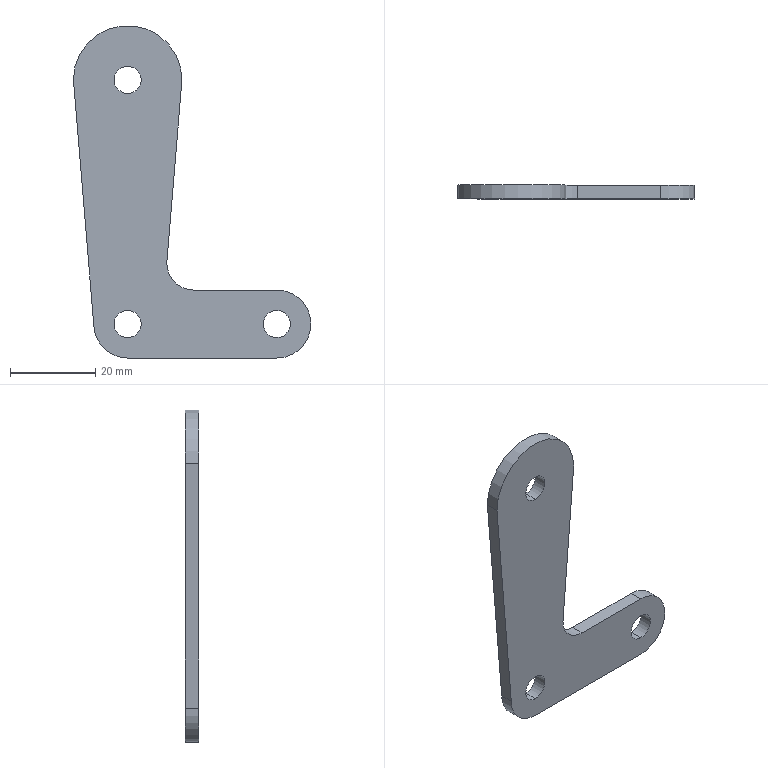Part | SolidWorks | features Extrusion 1 | 1 solid | 16 faces | box 55.575 x 3.175 x 77.8 mm | volume 6310 mm3 | cylinder 10 | plane 6 | commonest cylinder face diameters 6.35 x6 15.9 x2 12.7 x1 25.4 x1
STEP:
#1=CARTESIAN_POINT('',(34.925,3.175,-3.175));
#2=VERTEX_POINT('',#1);
#3=CARTESIAN_POINT('',(34.925,3.175,3.175));
#4=VERTEX_POINT('',#3);
#5=CARTESIAN_POINT('',(34.925,3.175,0.));
#6=DIRECTION('',(0.,1.,0.));
#7=DIRECTION('',(0.,0.,1.));
#8=AXIS2_PLACEMENT_3D('',#5,#6,#7);
#9=CIRCLE('',#8,3.175);
#10=EDGE_CURVE('',#2,#4,#9,.T.);
#11=ORIENTED_EDGE('',*,*,#10,.T.);
#12=CARTESIAN_POINT('',(34.925,0.,3.175));
#13=VERTEX_POINT('',#12);
#14=CARTESIAN_POINT('',(34.925,3.175,3.175));
#15=DIRECTION('',(0.,-1.,0.));
#16=VECTOR('',#15,1000.);
#17=LINE('',#14,#16);
#18=EDGE_CURVE('',#4,#13,#17,.T.);
#19=ORIENTED_EDGE('',*,*,#18,.T.);
#20=CARTESIAN_POINT('',(34.925,0.,-3.175));
#21=VERTEX_POINT('',#20);
#22=CARTESIAN_POINT('',(34.925,0.,0.));
#23=DIRECTION('',(0.,1.,0.));
#24=DIRECTION('',(0.,0.,1.));
#25=AXIS2_PLACEMENT_3D('',#22,#23,#24);
#26=CIRCLE('',#25,3.175);
#27=EDGE_CURVE('',#21,#13,#26,.T.);
#28=ORIENTED_EDGE('',*,*,#27,.F.);
#29=CARTESIAN_POINT('',(34.925,3.175,-3.175));
#30=DIRECTION('',(0.,-1.,0.));
#31=VECTOR('',#30,1000.);
#32=LINE('',#29,#31);
#33=EDGE_CURVE('',#2,#21,#32,.T.);
#34=ORIENTED_EDGE('',*,*,#33,.F.);
#35=EDGE_LOOP('',(#11,#19,#28,#34));
#36=FACE_OUTER_BOUND('',#35,.T.);
#37=CARTESIAN_POINT('',(34.925,3.175,0.));
#38=DIRECTION('',(0.,-1.,0.));
#39=DIRECTION('',(0.,0.,-1.));
#40=AXIS2_PLACEMENT_3D('',#37,#38,#39);
#41=CYLINDRICAL_SURFACE('',#40,3.175);
#42=ADVANCED_FACE('',(#36),#41,.F.);
#43=CARTESIAN_POINT('',(0.,3.175,53.975));
#44=VERTEX_POINT('',#43);
#45=CARTESIAN_POINT('',(0.,3.175,60.325));
#46=VERTEX_POINT('',#45);
#47=CARTESIAN_POINT('',(0.,3.175,57.15));
#48=DIRECTION('',(0.,1.,0.));
#49=DIRECTION('',(0.,0.,1.));
#50=AXIS2_PLACEMENT_3D('',#47,#48,#49);
#51=CIRCLE('',#50,3.175);
#52=EDGE_CURVE('',#44,#46,#51,.T.);
#53=ORIENTED_EDGE('',*,*,#52,.T.);
#54=CARTESIAN_POINT('',(0.,0.,60.325));
#55=VERTEX_POINT('',#54);
#56=CARTESIAN_POINT('',(0.,3.175,60.325));
#57=DIRECTION('',(0.,-1.,0.));
#58=VECTOR('',#57,1000.);
#59=LINE('',#56,#58);
#60=EDGE_CURVE('',#46,#55,#59,.T.);
#61=ORIENTED_EDGE('',*,*,#60,.T.);
#62=CARTESIAN_POINT('',(0.,0.,53.975));
#63=VERTEX_POINT('',#62);
#64=CARTESIAN_POINT('',(0.,0.,57.15));
#65=DIRECTION('',(0.,1.,0.));
#66=DIRECTION('',(0.,0.,1.));
#67=AXIS2_PLACEMENT_3D('',#64,#65,#66);
#68=CIRCLE('',#67,3.175);
#69=EDGE_CURVE('',#63,#55,#68,.T.);
#70=ORIENTED_EDGE('',*,*,#69,.F.);
#71=CARTESIAN_POINT('',(0.,3.175,53.975));
#72=DIRECTION('',(0.,-1.,0.));
#73=VECTOR('',#72,1000.);
#74=LINE('',#71,#73);
#75=EDGE_CURVE('',#44,#63,#74,.T.);
#76=ORIENTED_EDGE('',*,*,#75,.F.);
#77=EDGE_LOOP('',(#53,#61,#70,#76));
#78=FACE_OUTER_BOUND('',#77,.T.);
#79=CARTESIAN_POINT('',(0.,3.175,57.15));
#80=DIRECTION('',(0.,-1.,0.));
#81=DIRECTION('',(0.,0.,-1.));
#82=AXIS2_PLACEMENT_3D('',#79,#80,#81);
#83=CYLINDRICAL_SURFACE('',#82,3.175);
#84=ADVANCED_FACE('',(#78),#83,.F.);
#85=CARTESIAN_POINT('',(0.,3.175,-3.175));
#86=VERTEX_POINT('',#85);
#87=CARTESIAN_POINT('',(0.,3.175,3.175));
#88=VERTEX_POINT('',#87);
#89=CARTESIAN_POINT('',(0.,3.175,0.));
#90=DIRECTION('',(0.,1.,0.));
#91=DIRECTION('',(0.,0.,1.));
#92=AXIS2_PLACEMENT_3D('',#89,#90,#91);
#93=CIRCLE('',#92,3.175);
#94=EDGE_CURVE('',#86,#88,#93,.T.);
#95=ORIENTED_EDGE('',*,*,#94,.T.);
#96=CARTESIAN_POINT('',(0.,0.,3.175));
#97=VERTEX_POINT('',#96);
#98=CARTESIAN_POINT('',(0.,3.175,3.175));
#99=DIRECTION('',(0.,-1.,0.));
#100=VECTOR('',#99,1000.);
#101=LINE('',#98,#100);
#102=EDGE_CURVE('',#88,#97,#101,.T.);
#103=ORIENTED_EDGE('',*,*,#102,.T.);
#104=CARTESIAN_POINT('',(0.,0.,-3.175));
#105=VERTEX_POINT('',#104);
#106=CARTESIAN_POINT('',(0.,0.,0.));
#107=DIRECTION('',(0.,1.,0.));
#108=DIRECTION('',(0.,0.,1.));
#109=AXIS2_PLACEMENT_3D('',#106,#107,#108);
#110=CIRCLE('',#109,3.175);
#111=EDGE_CURVE('',#105,#97,#110,.T.);
#112=ORIENTED_EDGE('',*,*,#111,.F.);
#113=CARTESIAN_POINT('',(0.,3.175,-3.175));
#114=DIRECTION('',(0.,-1.,0.));
#115=VECTOR('',#114,1000.);
#116=LINE('',#113,#115);
#117=EDGE_CURVE('',#86,#105,#116,.T.);
#118=ORIENTED_EDGE('',*,*,#117,.F.);
#119=EDGE_LOOP('',(#95,#103,#112,#118));
#120=FACE_OUTER_BOUND('',#119,.T.);
#121=CARTESIAN_POINT('',(0.,3.175,0.));
#122=DIRECTION('',(0.,-1.,0.));
#123=DIRECTION('',(0.,0.,-1.));
#124=AXIS2_PLACEMENT_3D('',#121,#122,#123);
#125=CYLINDRICAL_SURFACE('',#124,3.175);
#126=ADVANCED_FACE('',(#120),#125,.F.);
#127=CARTESIAN_POINT('',(15.498,0.,7.95));
#128=VERTEX_POINT('',#127);
#129=CARTESIAN_POINT('',(9.149,0.,14.426));
#130=VERTEX_POINT('',#129);
#131=CARTESIAN_POINT('',(15.498,0.,14.3));
#132=DIRECTION('',(0.,1.,0.));
#133=DIRECTION('',(0.,0.,1.));
#134=AXIS2_PLACEMENT_3D('',#131,#132,#133);
#135=CIRCLE('',#134,6.35);
#136=EDGE_CURVE('',#128,#130,#135,.T.);
#137=ORIENTED_EDGE('',*,*,#136,.F.);
#138=CARTESIAN_POINT('',(15.498,3.175,7.95));
#139=VERTEX_POINT('',#138);
#140=CARTESIAN_POINT('',(15.498,3.175,7.95));
#141=DIRECTION('',(0.,-1.,0.));
#142=VECTOR('',#141,1000.);
#143=LINE('',#140,#142);
#144=EDGE_CURVE('',#139,#128,#143,.T.);
#145=ORIENTED_EDGE('',*,*,#144,.F.);
#146=CARTESIAN_POINT('',(9.149,3.175,14.426));
#147=VERTEX_POINT('',#146);
#148=CARTESIAN_POINT('',(15.498,3.175,14.3));
#149=DIRECTION('',(0.,1.,0.));
#150=DIRECTION('',(0.,0.,1.));
#151=AXIS2_PLACEMENT_3D('',#148,#149,#150);
#152=CIRCLE('',#151,6.35);
#153=EDGE_CURVE('',#139,#147,#152,.T.);
#154=ORIENTED_EDGE('',*,*,#153,.T.);
#155=CARTESIAN_POINT('',(9.149,3.175,14.426));
#156=DIRECTION('',(0.,-1.,0.));
#157=VECTOR('',#156,1000.);
#158=LINE('',#155,#157);
#159=EDGE_CURVE('',#147,#130,#158,.T.);
#160=ORIENTED_EDGE('',*,*,#159,.T.);
#161=EDGE_LOOP('',(#137,#145,#154,#160));
#162=FACE_OUTER_BOUND('',#161,.T.);
#163=CARTESIAN_POINT('',(15.498,3.175,14.3));
#164=DIRECTION('',(0.,-1.,0.));
#165=DIRECTION('',(0.,0.,-1.));
#166=AXIS2_PLACEMENT_3D('',#163,#164,#165);
#167=CYLINDRICAL_SURFACE('',#166,6.35);
#168=ADVANCED_FACE('',(#162),#167,.F.);
#169=CARTESIAN_POINT('',(34.925,0.,7.95));
#170=VERTEX_POINT('',#169);
#171=CARTESIAN_POINT('',(0.,0.,7.95));
#172=DIRECTION('',(-1.,0.,0.));
#173=VECTOR('',#172,1000.);
#174=LINE('',#171,#173);
#175=EDGE_CURVE('',#170,#128,#174,.T.);
#176=ORIENTED_EDGE('',*,*,#175,.F.);
#177=CARTESIAN_POINT('',(34.925,3.175,7.95));
#178=VERTEX_POINT('',#177);
#179=CARTESIAN_POINT('',(34.925,3.175,7.95));
#180=DIRECTION('',(0.,-1.,0.));
#181=VECTOR('',#180,1000.);
#182=LINE('',#179,#181);
#183=EDGE_CURVE('',#178,#170,#182,.T.);
#184=ORIENTED_EDGE('',*,*,#183,.F.);
#185=CARTESIAN_POINT('',(0.,3.175,7.95));
#186=DIRECTION('',(-1.,0.,0.));
#187=VECTOR('',#186,1000.);
#188=LINE('',#185,#187);
#189=EDGE_CURVE('',#178,#139,#188,.T.);
#190=ORIENTED_EDGE('',*,*,#189,.T.);
#191=ORIENTED_EDGE('',*,*,#144,.T.);
#192=EDGE_LOOP('',(#176,#184,#190,#191));
#193=FACE_OUTER_BOUND('',#192,.T.);
#194=CARTESIAN_POINT('',(0.,3.175,7.95));
#195=DIRECTION('',(0.,0.,1.));
#196=DIRECTION('',(1.,0.,0.));
#197=AXIS2_PLACEMENT_3D('',#194,#195,#196);
#198=PLANE('',#197);
#199=ADVANCED_FACE('',(#193),#198,.T.);
#200=CARTESIAN_POINT('',(34.925,0.,-7.95));
#201=VERTEX_POINT('',#200);
#202=CARTESIAN_POINT('',(34.925,0.,0.));
#203=DIRECTION('',(0.,-1.,0.));
#204=DIRECTION('',(0.,0.,1.));
#205=AXIS2_PLACEMENT_3D('',#202,#203,#204);
#206=CIRCLE('',#205,7.95);
#207=EDGE_CURVE('',#201,#170,#206,.T.);
#208=ORIENTED_EDGE('',*,*,#207,.F.);
#209=CARTESIAN_POINT('',(34.925,3.175,-7.95));
#210=VERTEX_POINT('',#209);
#211=CARTESIAN_POINT('',(34.925,3.175,-7.95));
#212=DIRECTION('',(0.,-1.,0.));
#213=VECTOR('',#212,1000.);
#214=LINE('',#211,#213);
#215=EDGE_CURVE('',#210,#201,#214,.T.);
#216=ORIENTED_EDGE('',*,*,#215,.F.);
#217=CARTESIAN_POINT('',(34.925,3.175,0.));
#218=DIRECTION('',(0.,-1.,0.));
#219=DIRECTION('',(0.,0.,1.));
#220=AXIS2_PLACEMENT_3D('',#217,#218,#219);
#221=CIRCLE('',#220,7.95);
#222=EDGE_CURVE('',#210,#178,#221,.T.);
#223=ORIENTED_EDGE('',*,*,#222,.T.);
#224=ORIENTED_EDGE('',*,*,#183,.T.);
#225=EDGE_LOOP('',(#208,#216,#223,#224));
#226=FACE_OUTER_BOUND('',#225,.T.);
#227=CARTESIAN_POINT('',(34.925,3.175,0.));
#228=DIRECTION('',(0.,-1.,0.));
#229=DIRECTION('',(0.,0.,-1.));
#230=AXIS2_PLACEMENT_3D('',#227,#228,#229);
#231=CYLINDRICAL_SURFACE('',#230,7.95);
#232=ADVANCED_FACE('',(#226),#231,.T.);
#233=CARTESIAN_POINT('',(0.,0.,-7.95));
#234=VERTEX_POINT('',#233);
#235=CARTESIAN_POINT('',(0.,0.,-7.95));
#236=DIRECTION('',(1.,0.,0.));
#237=VECTOR('',#236,1000.);
#238=LINE('',#235,#237);
#239=EDGE_CURVE('',#234,#201,#238,.T.);
#240=ORIENTED_EDGE('',*,*,#239,.F.);
#241=CARTESIAN_POINT('',(0.,3.175,-7.95));
#242=VERTEX_POINT('',#241);
#243=CARTESIAN_POINT('',(0.,3.175,-7.95));
#244=DIRECTION('',(0.,-1.,0.));
#245=VECTOR('',#244,1000.);
#246=LINE('',#243,#245);
#247=EDGE_CURVE('',#242,#234,#246,.T.);
#248=ORIENTED_EDGE('',*,*,#247,.F.);
#249=CARTESIAN_POINT('',(0.,3.175,-7.95));
#250=DIRECTION('',(1.,0.,0.));
#251=VECTOR('',#250,1000.);
#252=LINE('',#249,#251);
#253=EDGE_CURVE('',#242,#210,#252,.T.);
#254=ORIENTED_EDGE('',*,*,#253,.T.);
#255=ORIENTED_EDGE('',*,*,#215,.T.);
#256=EDGE_LOOP('',(#240,#248,#254,#255));
#257=FACE_OUTER_BOUND('',#256,.T.);
#258=CARTESIAN_POINT('',(0.,3.175,-7.95));
#259=DIRECTION('',(0.,0.,-1.));
#260=DIRECTION('',(-1.,0.,0.));
#261=AXIS2_PLACEMENT_3D('',#258,#259,#260);
#262=PLANE('',#261);
#263=ADVANCED_FACE('',(#257),#262,.T.);
#264=CARTESIAN_POINT('',(-7.95,0.,0.));
#265=VERTEX_POINT('',#264);
#266=CARTESIAN_POINT('',(0.,0.,0.));
#267=DIRECTION('',(0.,1.,0.));
#268=DIRECTION('',(0.,0.,1.));
#269=AXIS2_PLACEMENT_3D('',#266,#267,#268);
#270=CIRCLE('',#269,7.95);
#271=EDGE_CURVE('',#234,#265,#270,.T.);
#272=ORIENTED_EDGE('',*,*,#271,.T.);
#273=CARTESIAN_POINT('',(-7.95,3.175,0.));
#274=VERTEX_POINT('',#273);
#275=CARTESIAN_POINT('',(-7.95,3.175,0.));
#276=DIRECTION('',(0.,-1.,0.));
#277=VECTOR('',#276,1000.);
#278=LINE('',#275,#277);
#279=EDGE_CURVE('',#274,#265,#278,.T.);
#280=ORIENTED_EDGE('',*,*,#279,.F.);
#281=CARTESIAN_POINT('',(0.,3.175,0.));
#282=DIRECTION('',(0.,1.,0.));
#283=DIRECTION('',(0.,0.,1.));
#284=AXIS2_PLACEMENT_3D('',#281,#282,#283);
#285=CIRCLE('',#284,7.95);
#286=EDGE_CURVE('',#242,#274,#285,.T.);
#287=ORIENTED_EDGE('',*,*,#286,.F.);
#288=ORIENTED_EDGE('',*,*,#247,.T.);
#289=EDGE_LOOP('',(#272,#280,#287,#288));
#290=FACE_OUTER_BOUND('',#289,.T.);
#291=CARTESIAN_POINT('',(0.,3.175,0.));
#292=DIRECTION('',(0.,-1.,0.));
#293=DIRECTION('',(0.,0.,-1.));
#294=AXIS2_PLACEMENT_3D('',#291,#292,#293);
#295=CYLINDRICAL_SURFACE('',#294,7.95);
#296=ADVANCED_FACE('',(#290),#295,.T.);
#297=CARTESIAN_POINT('',(-12.7,0.,57.15));
#298=VERTEX_POINT('',#297);
#299=CARTESIAN_POINT('',(-7.896,0.,-0.6562));
#300=DIRECTION('',(-0.08283,0.,0.9966));
#301=VECTOR('',#300,1000.);
#302=LINE('',#299,#301);
#303=EDGE_CURVE('',#265,#298,#302,.T.);
#304=ORIENTED_EDGE('',*,*,#303,.T.);
#305=CARTESIAN_POINT('',(-12.7,3.175,57.15));
#306=VERTEX_POINT('',#305);
#307=CARTESIAN_POINT('',(-12.7,3.175,57.15));
#308=DIRECTION('',(0.,-1.,0.));
#309=VECTOR('',#308,1000.);
#310=LINE('',#307,#309);
#311=EDGE_CURVE('',#306,#298,#310,.T.);
#312=ORIENTED_EDGE('',*,*,#311,.F.);
#313=CARTESIAN_POINT('',(-7.896,3.175,-0.6562));
#314=DIRECTION('',(-0.08283,0.,0.9966));
#315=VECTOR('',#314,1000.);
#316=LINE('',#313,#315);
#317=EDGE_CURVE('',#274,#306,#316,.T.);
#318=ORIENTED_EDGE('',*,*,#317,.F.);
#319=ORIENTED_EDGE('',*,*,#279,.T.);
#320=EDGE_LOOP('',(#304,#312,#318,#319));
#321=FACE_OUTER_BOUND('',#320,.T.);
#322=CARTESIAN_POINT('',(-7.896,3.175,-0.6562));
#323=DIRECTION('',(0.9966,0.,0.08283));
#324=DIRECTION('',(0.08283,0.,-0.9966));
#325=AXIS2_PLACEMENT_3D('',#322,#323,#324);
#326=PLANE('',#325);
#327=ADVANCED_FACE('',(#321),#326,.F.);
#328=CARTESIAN_POINT('',(12.7,0.,57.15));
#329=VERTEX_POINT('',#328);
#330=CARTESIAN_POINT('',(0.,0.,57.15));
#331=DIRECTION('',(0.,1.,0.));
#332=DIRECTION('',(0.,0.,1.));
#333=AXIS2_PLACEMENT_3D('',#330,#331,#332);
#334=CIRCLE('',#333,12.7);
#335=EDGE_CURVE('',#298,#329,#334,.T.);
#336=ORIENTED_EDGE('',*,*,#335,.T.);
#337=CARTESIAN_POINT('',(12.7,3.175,57.15));
#338=VERTEX_POINT('',#337);
#339=CARTESIAN_POINT('',(12.7,3.175,57.15));
#340=DIRECTION('',(0.,-1.,0.));
#341=VECTOR('',#340,1000.);
#342=LINE('',#339,#341);
#343=EDGE_CURVE('',#338,#329,#342,.T.);
#344=ORIENTED_EDGE('',*,*,#343,.F.);
#345=CARTESIAN_POINT('',(0.,3.175,57.15));
#346=DIRECTION('',(0.,1.,0.));
#347=DIRECTION('',(0.,0.,1.));
#348=AXIS2_PLACEMENT_3D('',#345,#346,#347);
#349=CIRCLE('',#348,12.7);
#350=EDGE_CURVE('',#306,#338,#349,.T.);
#351=ORIENTED_EDGE('',*,*,#350,.F.);
#352=ORIENTED_EDGE('',*,*,#311,.T.);
#353=EDGE_LOOP('',(#336,#344,#351,#352));
#354=FACE_OUTER_BOUND('',#353,.T.);
#355=CARTESIAN_POINT('',(0.,3.175,57.15));
#356=DIRECTION('',(0.,-1.,0.));
#357=DIRECTION('',(0.,0.,-1.));
#358=AXIS2_PLACEMENT_3D('',#355,#356,#357);
#359=CYLINDRICAL_SURFACE('',#358,12.7);
#360=ADVANCED_FACE('',(#354),#359,.T.);
#361=ORIENTED_EDGE('',*,*,#102,.F.);
#362=CARTESIAN_POINT('',(0.,3.175,0.));
#363=DIRECTION('',(0.,1.,0.));
#364=DIRECTION('',(0.,0.,1.));
#365=AXIS2_PLACEMENT_3D('',#362,#363,#364);
#366=CIRCLE('',#365,3.175);
#367=EDGE_CURVE('',#88,#86,#366,.T.);
#368=ORIENTED_EDGE('',*,*,#367,.T.);
#369=ORIENTED_EDGE('',*,*,#117,.T.);
#370=CARTESIAN_POINT('',(0.,0.,0.));
#371=DIRECTION('',(0.,1.,0.));
#372=DIRECTION('',(0.,0.,1.));
#373=AXIS2_PLACEMENT_3D('',#370,#371,#372);
#374=CIRCLE('',#373,3.175);
#375=EDGE_CURVE('',#97,#105,#374,.T.);
#376=ORIENTED_EDGE('',*,*,#375,.F.);
#377=EDGE_LOOP('',(#361,#368,#369,#376));
#378=FACE_OUTER_BOUND('',#377,.T.);
#379=CARTESIAN_POINT('',(0.,3.175,0.));
#380=DIRECTION('',(0.,-1.,0.));
#381=DIRECTION('',(0.,0.,-1.));
#382=AXIS2_PLACEMENT_3D('',#379,#380,#381);
#383=CYLINDRICAL_SURFACE('',#382,3.175);
#384=ADVANCED_FACE('',(#378),#383,.F.);
#385=CARTESIAN_POINT('',(7.896,0.,-0.6562));
#386=DIRECTION('',(-0.08283,0.,-0.9966));
#387=VECTOR('',#386,1000.);
#388=LINE('',#385,#387);
#389=EDGE_CURVE('',#329,#130,#388,.T.);
#390=ORIENTED_EDGE('',*,*,#389,.T.);
#391=ORIENTED_EDGE('',*,*,#159,.F.);
#392=CARTESIAN_POINT('',(7.896,3.175,-0.6562));
#393=DIRECTION('',(-0.08283,0.,-0.9966));
#394=VECTOR('',#393,1000.);
#395=LINE('',#392,#394);
#396=EDGE_CURVE('',#338,#147,#395,.T.);
#397=ORIENTED_EDGE('',*,*,#396,.F.);
#398=ORIENTED_EDGE('',*,*,#343,.T.);
#399=EDGE_LOOP('',(#390,#391,#397,#398));
#400=FACE_OUTER_BOUND('',#399,.T.);
#401=CARTESIAN_POINT('',(7.896,3.175,-0.6562));
#402=DIRECTION('',(-0.9966,0.,0.08283));
#403=DIRECTION('',(0.08283,0.,0.9966));
#404=AXIS2_PLACEMENT_3D('',#401,#402,#403);
#405=PLANE('',#404);
#406=ADVANCED_FACE('',(#400),#405,.F.);
#407=ORIENTED_EDGE('',*,*,#60,.F.);
#408=CARTESIAN_POINT('',(0.,3.175,57.15));
#409=DIRECTION('',(0.,1.,0.));
#410=DIRECTION('',(0.,0.,1.));
#411=AXIS2_PLACEMENT_3D('',#408,#409,#410);
#412=CIRCLE('',#411,3.175);
#413=EDGE_CURVE('',#46,#44,#412,.T.);
#414=ORIENTED_EDGE('',*,*,#413,.T.);
#415=ORIENTED_EDGE('',*,*,#75,.T.);
#416=CARTESIAN_POINT('',(0.,0.,57.15));
#417=DIRECTION('',(0.,1.,0.));
#418=DIRECTION('',(0.,0.,1.));
#419=AXIS2_PLACEMENT_3D('',#416,#417,#418);
#420=CIRCLE('',#419,3.175);
#421=EDGE_CURVE('',#55,#63,#420,.T.);
#422=ORIENTED_EDGE('',*,*,#421,.F.);
#423=EDGE_LOOP('',(#407,#414,#415,#422));
#424=FACE_OUTER_BOUND('',#423,.T.);
#425=CARTESIAN_POINT('',(0.,3.175,57.15));
#426=DIRECTION('',(0.,-1.,0.));
#427=DIRECTION('',(0.,0.,-1.));
#428=AXIS2_PLACEMENT_3D('',#425,#426,#427);
#429=CYLINDRICAL_SURFACE('',#428,3.175);
#430=ADVANCED_FACE('',(#424),#429,.F.);
#431=ORIENTED_EDGE('',*,*,#18,.F.);
#432=CARTESIAN_POINT('',(34.925,3.175,0.));
#433=DIRECTION('',(0.,1.,0.));
#434=DIRECTION('',(0.,0.,1.));
#435=AXIS2_PLACEMENT_3D('',#432,#433,#434);
#436=CIRCLE('',#435,3.175);
#437=EDGE_CURVE('',#4,#2,#436,.T.);
#438=ORIENTED_EDGE('',*,*,#437,.T.);
#439=ORIENTED_EDGE('',*,*,#33,.T.);
#440=CARTESIAN_POINT('',(34.925,0.,0.));
#441=DIRECTION('',(0.,1.,0.));
#442=DIRECTION('',(0.,0.,1.));
#443=AXIS2_PLACEMENT_3D('',#440,#441,#442);
#444=CIRCLE('',#443,3.175);
#445=EDGE_CURVE('',#13,#21,#444,.T.);
#446=ORIENTED_EDGE('',*,*,#445,.F.);
#447=EDGE_LOOP('',(#431,#438,#439,#446));
#448=FACE_OUTER_BOUND('',#447,.T.);
#449=CARTESIAN_POINT('',(34.925,3.175,0.));
#450=DIRECTION('',(0.,-1.,0.));
#451=DIRECTION('',(0.,0.,-1.));
#452=AXIS2_PLACEMENT_3D('',#449,#450,#451);
#453=CYLINDRICAL_SURFACE('',#452,3.175);
#454=ADVANCED_FACE('',(#448),#453,.F.);
#455=ORIENTED_EDGE('',*,*,#52,.F.);
#456=ORIENTED_EDGE('',*,*,#413,.F.);
#457=EDGE_LOOP('',(#455,#456));
#458=FACE_BOUND('',#457,.T.);
#459=ORIENTED_EDGE('',*,*,#153,.F.);
#460=ORIENTED_EDGE('',*,*,#189,.F.);
#461=ORIENTED_EDGE('',*,*,#222,.F.);
#462=ORIENTED_EDGE('',*,*,#253,.F.);
#463=ORIENTED_EDGE('',*,*,#286,.T.);
#464=ORIENTED_EDGE('',*,*,#317,.T.);
#465=ORIENTED_EDGE('',*,*,#350,.T.);
#466=ORIENTED_EDGE('',*,*,#396,.T.);
#467=EDGE_LOOP('',(#459,#460,#461,#462,#463,#464,#465,#466));
#468=FACE_OUTER_BOUND('',#467,.T.);
#469=ORIENTED_EDGE('',*,*,#94,.F.);
#470=ORIENTED_EDGE('',*,*,#367,.F.);
#471=EDGE_LOOP('',(#469,#470));
#472=FACE_BOUND('',#471,.T.);
#473=ORIENTED_EDGE('',*,*,#10,.F.);
#474=ORIENTED_EDGE('',*,*,#437,.F.);
#475=EDGE_LOOP('',(#473,#474));
#476=FACE_BOUND('',#475,.T.);
#477=CARTESIAN_POINT('',(0.,3.175,0.));
#478=DIRECTION('',(0.,1.,0.));
#479=DIRECTION('',(0.,0.,1.));
#480=AXIS2_PLACEMENT_3D('',#477,#478,#479);
#481=PLANE('',#480);
#482=ADVANCED_FACE('',(#458,#468,#472,#476),#481,.T.);
#483=ORIENTED_EDGE('',*,*,#69,.T.);
#484=ORIENTED_EDGE('',*,*,#421,.T.);
#485=EDGE_LOOP('',(#483,#484));
#486=FACE_BOUND('',#485,.T.);
#487=ORIENTED_EDGE('',*,*,#136,.T.);
#488=ORIENTED_EDGE('',*,*,#389,.F.);
#489=ORIENTED_EDGE('',*,*,#335,.F.);
#490=ORIENTED_EDGE('',*,*,#303,.F.);
#491=ORIENTED_EDGE('',*,*,#271,.F.);
#492=ORIENTED_EDGE('',*,*,#239,.T.);
#493=ORIENTED_EDGE('',*,*,#207,.T.);
#494=ORIENTED_EDGE('',*,*,#175,.T.);
#495=EDGE_LOOP('',(#487,#488,#489,#490,#491,#492,#493,#494));
#496=FACE_OUTER_BOUND('',#495,.T.);
#497=ORIENTED_EDGE('',*,*,#111,.T.);
#498=ORIENTED_EDGE('',*,*,#375,.T.);
#499=EDGE_LOOP('',(#497,#498));
#500=FACE_BOUND('',#499,.T.);
#501=ORIENTED_EDGE('',*,*,#27,.T.);
#502=ORIENTED_EDGE('',*,*,#445,.T.);
#503=EDGE_LOOP('',(#501,#502));
#504=FACE_BOUND('',#503,.T.);
#505=CARTESIAN_POINT('',(0.,0.,0.));
#506=DIRECTION('',(0.,1.,0.));
#507=DIRECTION('',(0.,0.,1.));
#508=AXIS2_PLACEMENT_3D('',#505,#506,#507);
#509=PLANE('',#508);
#510=ADVANCED_FACE('',(#486,#496,#500,#504),#509,.F.);
#511=CLOSED_SHELL('',(#42,#84,#126,#168,#199,#232,#263,#296,#327,#360,#384,#406,#430,#454,#482,#510));
#512=MANIFOLD_SOLID_BREP('',#511);
#513=CARTESIAN_POINT('',(0.,0.,0.));
#514=DIRECTION('',(0.,0.,1.));
#515=DIRECTION('',(1.,0.,0.));
#516=AXIS2_PLACEMENT_3D('',#513,#514,#515);
#517=(LENGTH_UNIT()NAMED_UNIT(*)SI_UNIT(.MILLI.,.METRE.));
#518=UNCERTAINTY_MEASURE_WITH_UNIT(LENGTH_MEASURE(0.00001),#517,'','');
#519=(NAMED_UNIT(*)PLANE_ANGLE_UNIT()SI_UNIT($,.RADIAN.));
#520=(NAMED_UNIT(*)SI_UNIT($,.STERADIAN.)SOLID_ANGLE_UNIT());
#521=(GEOMETRIC_REPRESENTATION_CONTEXT(3)GLOBAL_UNCERTAINTY_ASSIGNED_CONTEXT((#518))GLOBAL_UNIT_ASSIGNED_CONTEXT((#517,#519,#520))REPRESENTATION_CONTEXT('',''));
#522=ADVANCED_BREP_SHAPE_REPRESENTATION('',(#512,#516),#521);